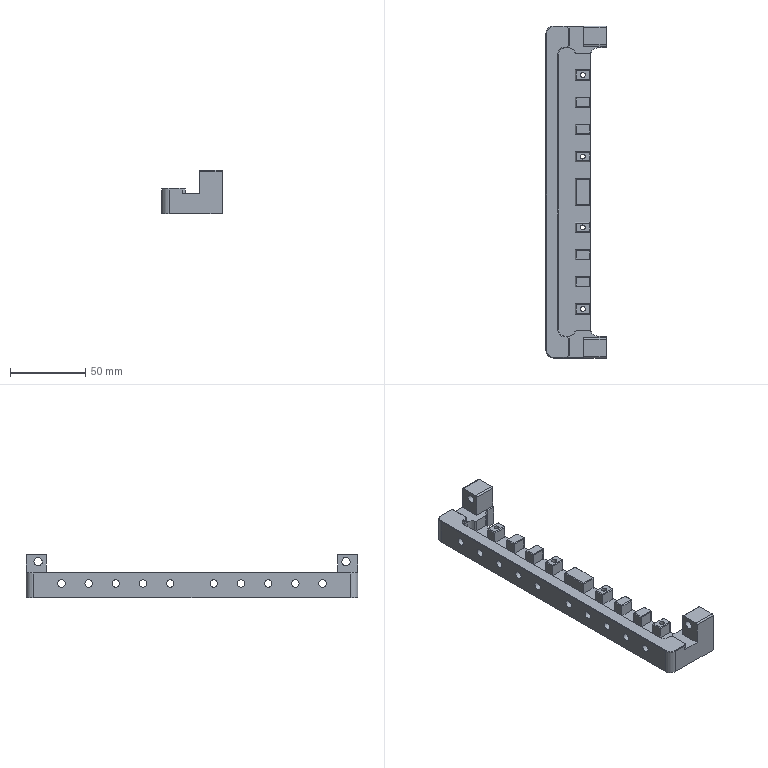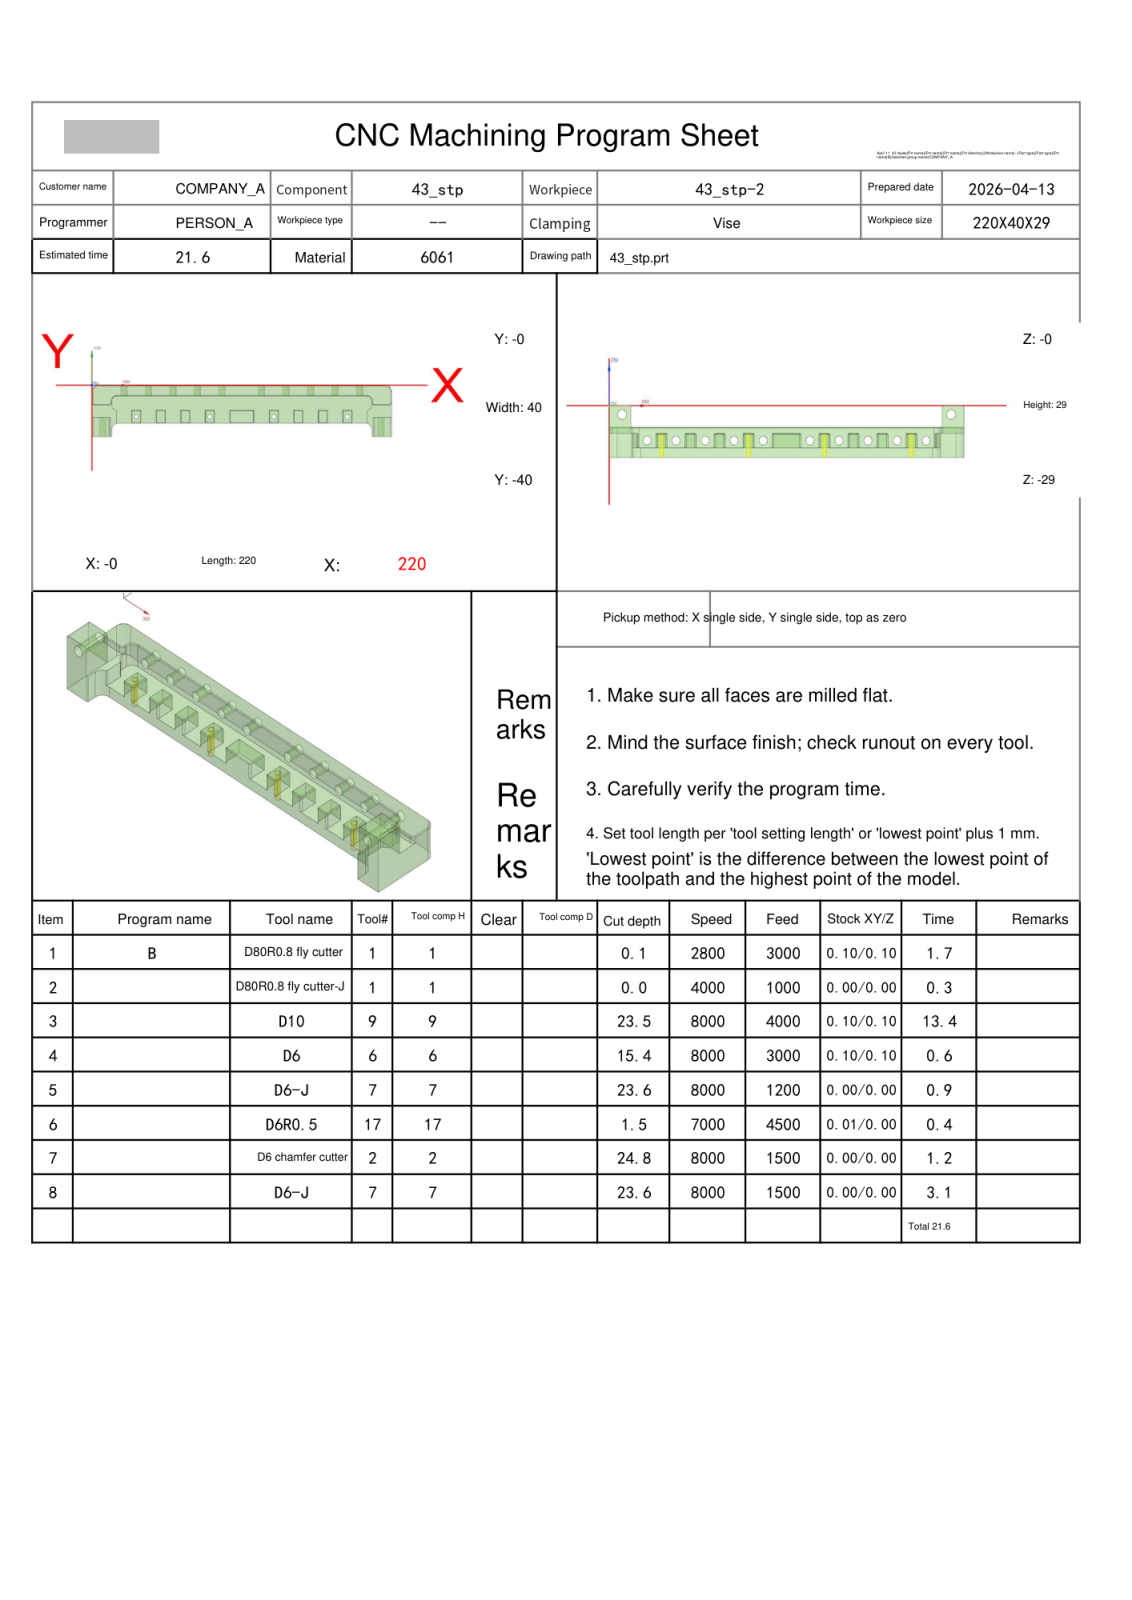NC program | NX | posted by the shop | part box 40 x 220 x 29 mm
Lines 1 to 134 of 14837:
%
O0001
(Machine time: 23.13 MIN)
(===Total Tool:6===)
(T1=D80R0.8 fly cutter D=80.  R=0.8  D-  H01 Z=-0.   )
(T9=D10     D=10.  R=0.   D-  H09 Z=-23.5 )
(T6=D6      D=6.   R=0.   D-  H06 Z=-15.4 )
(T7=D6-J    D=6.   R=0.   D-  H07 Z=-23.6 )
(T17=D6R0.5 D=6.   R=0.5  D-  H17 Z=-1.5  )
(T2=D6 chamfer cutter   D=6.   R=0.   D-  H02 Z=-24.8 )
G80 G90 G17 G49 G40
G91 G28 Z0
M01
N1 T01 M06
(D80R0.8 fly cutter  D=80. R=0.8 H=01 ce=0.10 di=0.10)
G00 G90 G54 X-52.097 Y-21.938 M03 S2800
G43 H01 Z20.
M08
Z7.325
G01 Z5.325 F3000.
X-40.097 Y-21.797
X260.097 Y-18.263
X272.097 Y-18.122
Z7.325
G00 X-52.097 Y-21.938
Z6.85
G01 Z4.85
X-40.097 Y-21.797
X260.097 Y-18.263
X272.097 Y-18.122
Z6.85
G00 X-52.097 Y-21.938
Z6.375
G01 Z4.375
X-40.097 Y-21.797
X260.097 Y-18.263
X272.097 Y-18.122
Z6.375
G00 X-52.097 Y-21.938
Z5.9
G01 Z3.9
X-40.097 Y-21.797
X260.097 Y-18.263
X272.097 Y-18.122
Z5.9
G00 Z20.
X-52.097 Y-21.938
Z5.425
G01 Z3.425
X-40.097 Y-21.797
X260.097 Y-18.263
X272.097 Y-18.122
Z5.425
G00 Z20.
X-52.097 Y-21.938
Z4.95
G01 Z2.95
X-40.097 Y-21.797
X260.097 Y-18.263
X272.097 Y-18.122
Z4.95
G00 Z20.
X-52.097 Y-21.938
Z4.475
G01 Z2.475
X-40.097 Y-21.797
X260.097 Y-18.263
X272.097 Y-18.122
Z4.475
G00 Z20.
X-52.097 Y-21.938
Z4.
G01 Z2.
X-40.097 Y-21.797
X260.097 Y-18.263
X272.097 Y-18.122
Z4.
G00 Z20.
X-52.097 Y-21.938
Z3.525
G01 Z1.525
X-40.097 Y-21.797
X260.097 Y-18.263
X272.097 Y-18.122
Z3.525
G00 Z20.
X-52.097 Y-21.938
Z3.05
G01 Z1.05
X-40.097 Y-21.797
X260.097 Y-18.263
X272.097 Y-18.122
Z3.05
G00 Z20.
X-52.097 Y-21.938
Z2.575
G01 Z.575
X-40.097 Y-21.797
X260.097 Y-18.263
X272.097 Y-18.122
Z2.575
G00 Z20.
X-52.097 Y-21.938
Z2.1
G01 Z.1
X-40.097 Y-21.797
X260.097 Y-18.263
X272.097 Y-18.122
Z2.1
G00 Z20.
G91 G28 Z0.0
M05
M09
G91 G28 Z0.0
M01
N2 T01 M06
(D80R0.8 fly cutter-J  D=80. R=0.8 H=01 ce=0.00 di=0.00)
G00 G90 G54 X-51.999 Y-21.938 M03 S4000
G43 H01 Z20.
M08
Z2.
G01 Z0.0 F1000.
X-39.999 Y-21.797
X259.999 Y-18.262
X271.999 Y-18.12
Z2.
G00 Z20.
G91 G28 Z0.0
M05
M09
G91 G28 Z0.0
M01